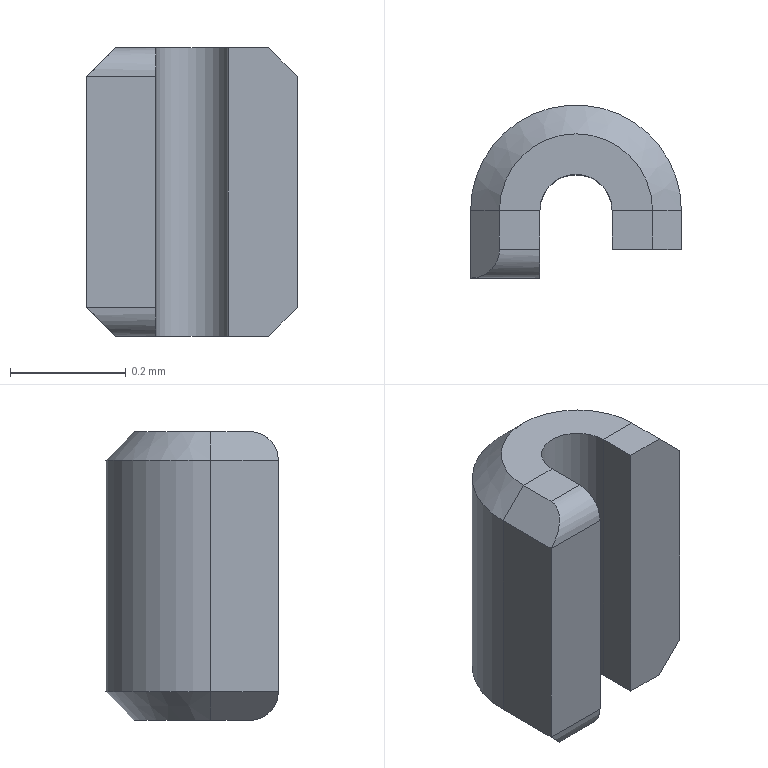Part | Creo | 1 solid | 22 faces | box 0.365 x 0.3 x 0.5 mm | volume 0.03234 mm3 | plane 16 | cylinder 4 | cone 2 | commonest cylinder face diameters 0.1 x2 0.125 x1 0.365 x1
STEP:
#1=CARTESIAN_POINT('',(0.,0.,0.));
#2=DIRECTION('',(0.,0.,1.));
#3=DIRECTION('',(1.,0.,0.));
#4=AXIS2_PLACEMENT_3D('',#1,#2,#3);
#5=CARTESIAN_POINT('',(-0.125,979.069,-1855.878));
#6=VERTEX_POINT('',#5);
#7=CARTESIAN_POINT('',(-0.195,979.069,-1855.878));
#8=VERTEX_POINT('',#7);
#9=CARTESIAN_POINT('',(-0.125,979.069,-1855.878));
#10=DIRECTION('',(-1.,0.,0.));
#11=VECTOR('',#10,0.07);
#12=LINE('',#9,#11);
#13=EDGE_CURVE('',#6,#8,#12,.T.);
#14=ORIENTED_EDGE('',*,*,#13,.F.);
#15=CARTESIAN_POINT('',(0.,979.069,-1855.878));
#16=VERTEX_POINT('',#15);
#17=CARTESIAN_POINT('',(-0.0625,979.069,-1855.878));
#18=DIRECTION('',(0.,0.,-1.));
#19=DIRECTION('',(-1.,0.,0.));
#20=AXIS2_PLACEMENT_3D('',#17,#18,#19);
#21=CIRCLE('',#20,0.0625);
#22=EDGE_CURVE('',#6,#16,#21,.T.);
#23=ORIENTED_EDGE('',*,*,#22,.T.);
#24=CARTESIAN_POINT('',(0.07,979.069,-1855.878));
#25=VERTEX_POINT('',#24);
#26=CARTESIAN_POINT('',(0.07,979.069,-1855.878));
#27=DIRECTION('',(-1.,0.,0.));
#28=VECTOR('',#27,0.07);
#29=LINE('',#26,#28);
#30=EDGE_CURVE('',#25,#16,#29,.T.);
#31=ORIENTED_EDGE('',*,*,#30,.F.);
#32=CARTESIAN_POINT('',(-0.0625,979.069,-1855.878));
#33=DIRECTION('',(0.,0.,1.));
#34=DIRECTION('',(1.,0.,0.));
#35=AXIS2_PLACEMENT_3D('',#32,#33,#34);
#36=CIRCLE('',#35,0.1325);
#37=EDGE_CURVE('',#25,#8,#36,.T.);
#38=ORIENTED_EDGE('',*,*,#37,.T.);
#39=EDGE_LOOP('',(#14,#23,#31,#38));
#40=FACE_OUTER_BOUND('',#39,.F.);
#41=CARTESIAN_POINT('',(-0.245,979.069,-1855.878));
#42=DIRECTION('',(0.,0.,-1.));
#43=DIRECTION('',(-1.,0.,0.));
#44=AXIS2_PLACEMENT_3D('',#41,#42,#43);
#45=PLANE('',#44);
#46=ADVANCED_FACE('',(#40),#45,.T.);
#47=CARTESIAN_POINT('',(-0.125,979.002,-1855.878));
#48=VERTEX_POINT('',#47);
#49=CARTESIAN_POINT('',(-0.125,979.002,-1855.878));
#50=DIRECTION('',(0.,1.,0.));
#51=VECTOR('',#50,0.0675);
#52=LINE('',#49,#51);
#53=EDGE_CURVE('',#48,#6,#52,.T.);
#54=ORIENTED_EDGE('',*,*,#53,.T.);
#55=ORIENTED_EDGE('',*,*,#13,.T.);
#56=CARTESIAN_POINT('',(-0.195,979.002,-1855.878));
#57=VERTEX_POINT('',#56);
#58=CARTESIAN_POINT('',(-0.195,979.069,-1855.878));
#59=DIRECTION('',(0.,-1.,0.));
#60=VECTOR('',#59,0.0675);
#61=LINE('',#58,#60);
#62=EDGE_CURVE('',#8,#57,#61,.T.);
#63=ORIENTED_EDGE('',*,*,#62,.T.);
#64=CARTESIAN_POINT('',(-0.125,979.002,-1855.878));
#65=DIRECTION('',(-1.,0.,0.));
#66=VECTOR('',#65,0.07);
#67=LINE('',#64,#66);
#68=EDGE_CURVE('',#48,#57,#67,.T.);
#69=ORIENTED_EDGE('',*,*,#68,.F.);
#70=EDGE_LOOP('',(#54,#55,#63,#69));
#71=FACE_OUTER_BOUND('',#70,.F.);
#72=CARTESIAN_POINT('',(0.,979.069,-1855.878));
#73=DIRECTION('',(0.,0.,-1.));
#74=DIRECTION('',(-1.,0.,0.));
#75=AXIS2_PLACEMENT_3D('',#72,#73,#74);
#76=PLANE('',#75);
#77=ADVANCED_FACE('',(#71),#76,.T.);
#78=CARTESIAN_POINT('',(-0.125,979.069,-1855.378));
#79=VERTEX_POINT('',#78);
#80=CARTESIAN_POINT('',(-0.125,979.002,-1855.378));
#81=VERTEX_POINT('',#80);
#82=CARTESIAN_POINT('',(-0.125,979.069,-1855.378));
#83=DIRECTION('',(0.,-1.,0.));
#84=VECTOR('',#83,0.0675);
#85=LINE('',#82,#84);
#86=EDGE_CURVE('',#79,#81,#85,.T.);
#87=ORIENTED_EDGE('',*,*,#86,.F.);
#88=CARTESIAN_POINT('',(-0.125,979.069,-1855.878));
#89=DIRECTION('',(0.,0.,1.));
#90=VECTOR('',#89,0.5);
#91=LINE('',#88,#90);
#92=EDGE_CURVE('',#6,#79,#91,.T.);
#93=ORIENTED_EDGE('',*,*,#92,.F.);
#94=ORIENTED_EDGE('',*,*,#53,.F.);
#95=CARTESIAN_POINT('',(-0.125,978.952,-1855.828));
#96=VERTEX_POINT('',#95);
#97=CARTESIAN_POINT('',(-0.125,979.002,-1855.828));
#98=DIRECTION('',(-1.,0.,0.));
#99=DIRECTION('',(0.,0.,-1.));
#100=AXIS2_PLACEMENT_3D('',#97,#98,#99);
#101=CIRCLE('',#100,0.05);
#102=EDGE_CURVE('',#48,#96,#101,.T.);
#103=ORIENTED_EDGE('',*,*,#102,.T.);
#104=CARTESIAN_POINT('',(-0.125,978.952,-1855.428));
#105=VERTEX_POINT('',#104);
#106=CARTESIAN_POINT('',(-0.125,978.952,-1855.828));
#107=DIRECTION('',(0.,0.,1.));
#108=VECTOR('',#107,0.4);
#109=LINE('',#106,#108);
#110=EDGE_CURVE('',#96,#105,#109,.T.);
#111=ORIENTED_EDGE('',*,*,#110,.T.);
#112=CARTESIAN_POINT('',(-0.125,979.002,-1855.428));
#113=DIRECTION('',(-1.,0.,0.));
#114=DIRECTION('',(0.,-1.,0.));
#115=AXIS2_PLACEMENT_3D('',#112,#113,#114);
#116=CIRCLE('',#115,0.05);
#117=EDGE_CURVE('',#105,#81,#116,.T.);
#118=ORIENTED_EDGE('',*,*,#117,.T.);
#119=EDGE_LOOP('',(#87,#93,#94,#103,#111,#118));
#120=FACE_OUTER_BOUND('',#119,.F.);
#121=CARTESIAN_POINT('',(-0.125,979.069,-1854.906));
#122=DIRECTION('',(1.,0.,0.));
#123=DIRECTION('',(0.,0.,-1.));
#124=AXIS2_PLACEMENT_3D('',#121,#122,#123);
#125=PLANE('',#124);
#126=ADVANCED_FACE('',(#120),#125,.T.);
#127=CARTESIAN_POINT('',(-0.195,979.002,-1855.378));
#128=VERTEX_POINT('',#127);
#129=CARTESIAN_POINT('',(-0.195,979.069,-1855.378));
#130=VERTEX_POINT('',#129);
#131=CARTESIAN_POINT('',(-0.195,979.002,-1855.378));
#132=DIRECTION('',(0.,1.,0.));
#133=VECTOR('',#132,0.0675);
#134=LINE('',#131,#133);
#135=EDGE_CURVE('',#128,#130,#134,.T.);
#136=ORIENTED_EDGE('',*,*,#135,.T.);
#137=CARTESIAN_POINT('',(-0.195,979.069,-1855.378));
#138=DIRECTION('',(1.,0.,0.));
#139=VECTOR('',#138,0.07);
#140=LINE('',#137,#139);
#141=EDGE_CURVE('',#130,#79,#140,.T.);
#142=ORIENTED_EDGE('',*,*,#141,.T.);
#143=ORIENTED_EDGE('',*,*,#86,.T.);
#144=CARTESIAN_POINT('',(-0.195,979.002,-1855.378));
#145=DIRECTION('',(1.,0.,0.));
#146=VECTOR('',#145,0.07);
#147=LINE('',#144,#146);
#148=EDGE_CURVE('',#128,#81,#147,.T.);
#149=ORIENTED_EDGE('',*,*,#148,.F.);
#150=EDGE_LOOP('',(#136,#142,#143,#149));
#151=FACE_OUTER_BOUND('',#150,.F.);
#152=CARTESIAN_POINT('',(-0.125,979.069,-1855.378));
#153=DIRECTION('',(0.,0.,-1.));
#154=DIRECTION('',(0.,1.,0.));
#155=AXIS2_PLACEMENT_3D('',#152,#153,#154);
#156=PLANE('',#155);
#157=ADVANCED_FACE('',(#151),#156,.F.);
#158=CARTESIAN_POINT('',(-0.245,979.069,-1855.428));
#159=VERTEX_POINT('',#158);
#160=CARTESIAN_POINT('',(-0.245,978.952,-1855.428));
#161=VERTEX_POINT('',#160);
#162=CARTESIAN_POINT('',(-0.245,979.069,-1855.428));
#163=DIRECTION('',(0.,-1.,0.));
#164=VECTOR('',#163,0.1175);
#165=LINE('',#162,#164);
#166=EDGE_CURVE('',#159,#161,#165,.T.);
#167=ORIENTED_EDGE('',*,*,#166,.F.);
#168=CARTESIAN_POINT('',(-0.195,979.069,-1855.378));
#169=DIRECTION('',(-0.7071,0.,-0.7071));
#170=VECTOR('',#169,0.07071);
#171=LINE('',#168,#170);
#172=EDGE_CURVE('',#130,#159,#171,.T.);
#173=ORIENTED_EDGE('',*,*,#172,.F.);
#174=ORIENTED_EDGE('',*,*,#135,.F.);
#175=CARTESIAN_POINT('',(-0.195,979.002,-1855.378));
#176=CARTESIAN_POINT('',(-0.195,978.997,-1855.378));
#177=CARTESIAN_POINT('',(-0.1964,978.988,-1855.38));
#178=CARTESIAN_POINT('',(-0.2002,978.979,-1855.384));
#179=CARTESIAN_POINT('',(-0.2052,978.971,-1855.389));
#180=CARTESIAN_POINT('',(-0.2133,978.962,-1855.397));
#181=CARTESIAN_POINT('',(-0.2256,978.954,-1855.409));
#182=CARTESIAN_POINT('',(-0.2379,978.952,-1855.421));
#183=CARTESIAN_POINT('',(-0.245,978.952,-1855.428));
#184=B_SPLINE_CURVE_WITH_KNOTS('',3,(#175,#176,#177,#178,#179,#180,#181,#182,#183),.UNSPECIFIED.,.F.,.F.,(4,1,1,1,1,1,4),(0.,0.125,0.25,0.375,0.5,0.75,1.),.UNSPECIFIED.);
#185=EDGE_CURVE('',#128,#161,#184,.T.);
#186=ORIENTED_EDGE('',*,*,#185,.T.);
#187=EDGE_LOOP('',(#167,#173,#174,#186));
#188=FACE_OUTER_BOUND('',#187,.F.);
#189=CARTESIAN_POINT('',(-0.245,979.069,-1855.428));
#190=DIRECTION('',(0.7071,0.,-0.7071));
#191=DIRECTION('',(-0.7071,0.,-0.7071));
#192=AXIS2_PLACEMENT_3D('',#189,#190,#191);
#193=PLANE('',#192);
#194=ADVANCED_FACE('',(#188),#193,.F.);
#195=CARTESIAN_POINT('',(-0.245,978.952,-1855.828));
#196=VERTEX_POINT('',#195);
#197=CARTESIAN_POINT('',(-0.245,978.952,-1855.828));
#198=DIRECTION('',(0.,0.,1.));
#199=VECTOR('',#198,0.4);
#200=LINE('',#197,#199);
#201=EDGE_CURVE('',#196,#161,#200,.T.);
#202=ORIENTED_EDGE('',*,*,#201,.F.);
#203=CARTESIAN_POINT('',(-0.245,979.069,-1855.828));
#204=VERTEX_POINT('',#203);
#205=CARTESIAN_POINT('',(-0.245,978.952,-1855.828));
#206=DIRECTION('',(0.,1.,0.));
#207=VECTOR('',#206,0.1175);
#208=LINE('',#205,#207);
#209=EDGE_CURVE('',#196,#204,#208,.T.);
#210=ORIENTED_EDGE('',*,*,#209,.T.);
#211=CARTESIAN_POINT('',(-0.245,979.069,-1855.428));
#212=DIRECTION('',(0.,0.,-1.));
#213=VECTOR('',#212,0.4);
#214=LINE('',#211,#213);
#215=EDGE_CURVE('',#159,#204,#214,.T.);
#216=ORIENTED_EDGE('',*,*,#215,.F.);
#217=ORIENTED_EDGE('',*,*,#166,.T.);
#218=EDGE_LOOP('',(#202,#210,#216,#217));
#219=FACE_OUTER_BOUND('',#218,.F.);
#220=CARTESIAN_POINT('',(-0.245,979.069,-1854.906));
#221=DIRECTION('',(1.,0.,0.));
#222=DIRECTION('',(0.,0.,-1.));
#223=AXIS2_PLACEMENT_3D('',#220,#221,#222);
#224=PLANE('',#223);
#225=ADVANCED_FACE('',(#219),#224,.F.);
#226=ORIENTED_EDGE('',*,*,#110,.F.);
#227=CARTESIAN_POINT('',(-0.245,978.952,-1855.828));
#228=DIRECTION('',(1.,0.,0.));
#229=VECTOR('',#228,0.12);
#230=LINE('',#227,#229);
#231=EDGE_CURVE('',#196,#96,#230,.T.);
#232=ORIENTED_EDGE('',*,*,#231,.F.);
#233=ORIENTED_EDGE('',*,*,#201,.T.);
#234=CARTESIAN_POINT('',(-0.125,978.952,-1855.428));
#235=DIRECTION('',(-1.,0.,0.));
#236=VECTOR('',#235,0.12);
#237=LINE('',#234,#236);
#238=EDGE_CURVE('',#105,#161,#237,.T.);
#239=ORIENTED_EDGE('',*,*,#238,.F.);
#240=EDGE_LOOP('',(#226,#232,#233,#239));
#241=FACE_OUTER_BOUND('',#240,.F.);
#242=CARTESIAN_POINT('',(-0.245,978.952,-1854.906));
#243=DIRECTION('',(0.,1.,0.));
#244=DIRECTION('',(0.,0.,1.));
#245=AXIS2_PLACEMENT_3D('',#242,#243,#244);
#246=PLANE('',#245);
#247=ADVANCED_FACE('',(#241),#246,.F.);
#248=CARTESIAN_POINT('',(-0.195,979.002,-1855.878));
#249=CARTESIAN_POINT('',(-0.195,978.997,-1855.878));
#250=CARTESIAN_POINT('',(-0.1964,978.988,-1855.877));
#251=CARTESIAN_POINT('',(-0.2002,978.979,-1855.873));
#252=CARTESIAN_POINT('',(-0.2052,978.971,-1855.868));
#253=CARTESIAN_POINT('',(-0.2133,978.962,-1855.86));
#254=CARTESIAN_POINT('',(-0.2256,978.954,-1855.848));
#255=CARTESIAN_POINT('',(-0.2379,978.952,-1855.835));
#256=CARTESIAN_POINT('',(-0.245,978.952,-1855.828));
#257=B_SPLINE_CURVE_WITH_KNOTS('',3,(#248,#249,#250,#251,#252,#253,#254,#255,#256),.UNSPECIFIED.,.F.,.F.,(4,1,1,1,1,1,4),(0.,0.125,0.25,0.375,0.5,0.75,1.),.UNSPECIFIED.);
#258=EDGE_CURVE('',#57,#196,#257,.T.);
#259=ORIENTED_EDGE('',*,*,#258,.T.);
#260=ORIENTED_EDGE('',*,*,#231,.T.);
#261=ORIENTED_EDGE('',*,*,#102,.F.);
#262=ORIENTED_EDGE('',*,*,#68,.T.);
#263=EDGE_LOOP('',(#259,#260,#261,#262));
#264=FACE_OUTER_BOUND('',#263,.F.);
#265=CARTESIAN_POINT('',(-0.245,979.002,-1855.828));
#266=DIRECTION('',(-1.,0.,0.));
#267=DIRECTION('',(0.,0.,1.));
#268=AXIS2_PLACEMENT_3D('',#265,#266,#267);
#269=CYLINDRICAL_SURFACE('',#268,0.05);
#270=ADVANCED_FACE('',(#264),#269,.T.);
#271=ORIENTED_EDGE('',*,*,#62,.F.);
#272=CARTESIAN_POINT('',(-0.245,979.069,-1855.828));
#273=DIRECTION('',(0.7071,0.,-0.7071));
#274=VECTOR('',#273,0.07071);
#275=LINE('',#272,#274);
#276=EDGE_CURVE('',#204,#8,#275,.T.);
#277=ORIENTED_EDGE('',*,*,#276,.F.);
#278=ORIENTED_EDGE('',*,*,#209,.F.);
#279=ORIENTED_EDGE('',*,*,#258,.F.);
#280=EDGE_LOOP('',(#271,#277,#278,#279));
#281=FACE_OUTER_BOUND('',#280,.F.);
#282=CARTESIAN_POINT('',(-0.245,979.069,-1855.828));
#283=DIRECTION('',(-0.7071,0.,-0.7071));
#284=DIRECTION('',(-0.7071,0.,0.7071));
#285=AXIS2_PLACEMENT_3D('',#282,#283,#284);
#286=PLANE('',#285);
#287=ADVANCED_FACE('',(#281),#286,.T.);
#288=ORIENTED_EDGE('',*,*,#276,.T.);
#289=ORIENTED_EDGE('',*,*,#37,.F.);
#290=CARTESIAN_POINT('',(0.12,979.069,-1855.828));
#291=VERTEX_POINT('',#290);
#292=CARTESIAN_POINT('',(0.07,979.069,-1855.878));
#293=DIRECTION('',(0.7071,0.,0.7071));
#294=VECTOR('',#293,0.07071);
#295=LINE('',#292,#294);
#296=EDGE_CURVE('',#25,#291,#295,.T.);
#297=ORIENTED_EDGE('',*,*,#296,.T.);
#298=CARTESIAN_POINT('',(-0.0625,979.069,-1855.828));
#299=DIRECTION('',(0.,0.,1.));
#300=DIRECTION('',(1.,0.,0.));
#301=AXIS2_PLACEMENT_3D('',#298,#299,#300);
#302=CIRCLE('',#301,0.1825);
#303=EDGE_CURVE('',#291,#204,#302,.T.);
#304=ORIENTED_EDGE('',*,*,#303,.T.);
#305=EDGE_LOOP('',(#288,#289,#297,#304));
#306=FACE_OUTER_BOUND('',#305,.F.);
#307=CARTESIAN_POINT('',(-0.0625,979.069,-1855.853));
#308=DIRECTION('',(0.,0.,1.));
#309=DIRECTION('',(1.,0.,0.));
#310=AXIS2_PLACEMENT_3D('',#307,#308,#309);
#311=CONICAL_SURFACE('',#310,0.1575,45.);
#312=ADVANCED_FACE('',(#306),#311,.T.);
#313=CARTESIAN_POINT('',(0.12,979.002,-1855.828));
#314=VERTEX_POINT('',#313);
#315=CARTESIAN_POINT('',(0.07,979.002,-1855.878));
#316=VERTEX_POINT('',#315);
#317=CARTESIAN_POINT('',(0.12,979.002,-1855.828));
#318=DIRECTION('',(-0.7071,0.,-0.7071));
#319=VECTOR('',#318,0.07071);
#320=LINE('',#317,#319);
#321=EDGE_CURVE('',#314,#316,#320,.T.);
#322=ORIENTED_EDGE('',*,*,#321,.F.);
#323=CARTESIAN_POINT('',(0.12,979.069,-1855.828));
#324=DIRECTION('',(0.,-1.,0.));
#325=VECTOR('',#324,0.0675);
#326=LINE('',#323,#325);
#327=EDGE_CURVE('',#291,#314,#326,.T.);
#328=ORIENTED_EDGE('',*,*,#327,.F.);
#329=ORIENTED_EDGE('',*,*,#296,.F.);
#330=CARTESIAN_POINT('',(0.07,979.002,-1855.878));
#331=DIRECTION('',(0.,1.,0.));
#332=VECTOR('',#331,0.0675);
#333=LINE('',#330,#332);
#334=EDGE_CURVE('',#316,#25,#333,.T.);
#335=ORIENTED_EDGE('',*,*,#334,.F.);
#336=EDGE_LOOP('',(#322,#328,#329,#335));
#337=FACE_OUTER_BOUND('',#336,.F.);
#338=CARTESIAN_POINT('',(0.12,979.002,-1855.828));
#339=DIRECTION('',(-0.7071,0.,0.7071));
#340=DIRECTION('',(0.7071,0.,0.7071));
#341=AXIS2_PLACEMENT_3D('',#338,#339,#340);
#342=PLANE('',#341);
#343=ADVANCED_FACE('',(#337),#342,.F.);
#344=CARTESIAN_POINT('',(0.12,979.002,-1855.428));
#345=VERTEX_POINT('',#344);
#346=CARTESIAN_POINT('',(0.12,979.002,-1855.828));
#347=DIRECTION('',(0.,0.,1.));
#348=VECTOR('',#347,0.4);
#349=LINE('',#346,#348);
#350=EDGE_CURVE('',#314,#345,#349,.T.);
#351=ORIENTED_EDGE('',*,*,#350,.F.);
#352=ORIENTED_EDGE('',*,*,#321,.T.);
#353=CARTESIAN_POINT('',(0.,979.002,-1855.878));
#354=VERTEX_POINT('',#353);
#355=CARTESIAN_POINT('',(0.07,979.002,-1855.878));
#356=DIRECTION('',(-1.,0.,0.));
#357=VECTOR('',#356,0.07);
#358=LINE('',#355,#357);
#359=EDGE_CURVE('',#316,#354,#358,.T.);
#360=ORIENTED_EDGE('',*,*,#359,.T.);
#361=CARTESIAN_POINT('',(0.,979.002,-1855.378));
#362=VERTEX_POINT('',#361);
#363=CARTESIAN_POINT('',(0.,979.002,-1855.878));
#364=DIRECTION('',(0.,0.,1.));
#365=VECTOR('',#364,0.5);
#366=LINE('',#363,#365);
#367=EDGE_CURVE('',#354,#362,#366,.T.);
#368=ORIENTED_EDGE('',*,*,#367,.T.);
#369=CARTESIAN_POINT('',(0.07,979.002,-1855.378));
#370=VERTEX_POINT('',#369);
#371=CARTESIAN_POINT('',(0.,979.002,-1855.378));
#372=DIRECTION('',(1.,0.,0.));
#373=VECTOR('',#372,0.07);
#374=LINE('',#371,#373);
#375=EDGE_CURVE('',#362,#370,#374,.T.);
#376=ORIENTED_EDGE('',*,*,#375,.T.);
#377=CARTESIAN_POINT('',(0.07,979.002,-1855.378));
#378=DIRECTION('',(0.7071,0.,-0.7071));
#379=VECTOR('',#378,0.07071);
#380=LINE('',#377,#379);
#381=EDGE_CURVE('',#370,#345,#380,.T.);
#382=ORIENTED_EDGE('',*,*,#381,.T.);
#383=EDGE_LOOP('',(#351,#352,#360,#368,#376,#382));
#384=FACE_OUTER_BOUND('',#383,.F.);
#385=CARTESIAN_POINT('',(0.,979.002,-1854.906));
#386=DIRECTION('',(0.,1.,0.));
#387=DIRECTION('',(0.,0.,1.));
#388=AXIS2_PLACEMENT_3D('',#385,#386,#387);
#389=PLANE('',#388);
#390=ADVANCED_FACE('',(#384),#389,.F.);
#391=CARTESIAN_POINT('',(0.12,979.069,-1855.428));
#392=VERTEX_POINT('',#391);
#393=CARTESIAN_POINT('',(0.12,979.069,-1855.828));
#394=DIRECTION('',(0.,0.,1.));
#395=VECTOR('',#394,0.4);
#396=LINE('',#393,#395);
#397=EDGE_CURVE('',#291,#392,#396,.T.);
#398=ORIENTED_EDGE('',*,*,#397,.F.);
#399=ORIENTED_EDGE('',*,*,#327,.T.);
#400=ORIENTED_EDGE('',*,*,#350,.T.);
#401=CARTESIAN_POINT('',(0.12,979.002,-1855.428));
#402=DIRECTION('',(0.,1.,0.));
#403=VECTOR('',#402,0.0675);
#404=LINE('',#401,#403);
#405=EDGE_CURVE('',#345,#392,#404,.T.);
#406=ORIENTED_EDGE('',*,*,#405,.T.);
#407=EDGE_LOOP('',(#398,#399,#400,#406));
#408=FACE_OUTER_BOUND('',#407,.F.);
#409=CARTESIAN_POINT('',(0.12,979.002,-1854.906));
#410=DIRECTION('',(-1.,0.,0.));
#411=DIRECTION('',(0.,0.,1.));
#412=AXIS2_PLACEMENT_3D('',#409,#410,#411);
#413=PLANE('',#412);
#414=ADVANCED_FACE('',(#408),#413,.F.);
#415=ORIENTED_EDGE('',*,*,#215,.T.);
#416=ORIENTED_EDGE('',*,*,#303,.F.);
#417=ORIENTED_EDGE('',*,*,#397,.T.);
#418=CARTESIAN_POINT('',(-0.0625,979.069,-1855.428));
#419=DIRECTION('',(0.,0.,-1.));
#420=DIRECTION('',(-1.,0.,0.));
#421=AXIS2_PLACEMENT_3D('',#418,#419,#420);
#422=CIRCLE('',#421,0.1825);
#423=EDGE_CURVE('',#159,#392,#422,.T.);
#424=ORIENTED_EDGE('',*,*,#423,.F.);
#425=EDGE_LOOP('',(#415,#416,#417,#424));
#426=FACE_OUTER_BOUND('',#425,.F.);
#427=CARTESIAN_POINT('',(-0.0625,979.069,-1854.906));
#428=DIRECTION('',(0.,0.,-1.));
#429=DIRECTION('',(-1.,0.,0.));
#430=AXIS2_PLACEMENT_3D('',#427,#428,#429);
#431=CYLINDRICAL_SURFACE('',#430,0.1825);
#432=ADVANCED_FACE('',(#426),#431,.T.);
#433=ORIENTED_EDGE('',*,*,#172,.T.);
#434=ORIENTED_EDGE('',*,*,#423,.T.);
#435=CARTESIAN_POINT('',(0.07,979.069,-1855.378));
#436=VERTEX_POINT('',#435);
#437=CARTESIAN_POINT('',(0.12,979.069,-1855.428));
#438=DIRECTION('',(-0.7071,0.,0.7071));
#439=VECTOR('',#438,0.07071);
#440=LINE('',#437,#439);
#441=EDGE_CURVE('',#392,#436,#440,.T.);
#442=ORIENTED_EDGE('',*,*,#441,.T.);
#443=CARTESIAN_POINT('',(-0.0625,979.069,-1855.378));
#444=DIRECTION('',(0.,0.,-1.));
#445=DIRECTION('',(-1.,0.,0.));
#446=AXIS2_PLACEMENT_3D('',#443,#444,#445);
#447=CIRCLE('',#446,0.1325);
#448=EDGE_CURVE('',#130,#436,#447,.T.);
#449=ORIENTED_EDGE('',*,*,#448,.F.);
#450=EDGE_LOOP('',(#433,#434,#442,#449));
#451=FACE_OUTER_BOUND('',#450,.F.);
#452=CARTESIAN_POINT('',(-0.0625,979.069,-1855.403));
#453=DIRECTION('',(0.,0.,-1.));
#454=DIRECTION('',(-1.,0.,0.));
#455=AXIS2_PLACEMENT_3D('',#452,#453,#454);
#456=CONICAL_SURFACE('',#455,0.1575,45.);
#457=ADVANCED_FACE('',(#451),#456,.T.);
#458=ORIENTED_EDGE('',*,*,#441,.F.);
#459=ORIENTED_EDGE('',*,*,#405,.F.);
#460=ORIENTED_EDGE('',*,*,#381,.F.);
#461=CARTESIAN_POINT('',(0.07,979.069,-1855.378));
#462=DIRECTION('',(0.,-1.,0.));
#463=VECTOR('',#462,0.0675);
#464=LINE('',#461,#463);
#465=EDGE_CURVE('',#436,#370,#464,.T.);
#466=ORIENTED_EDGE('',*,*,#465,.F.);
#467=EDGE_LOOP('',(#458,#459,#460,#466));
#468=FACE_OUTER_BOUND('',#467,.F.);
#469=CARTESIAN_POINT('',(0.12,979.002,-1855.428));
#470=DIRECTION('',(-0.7071,0.,-0.7071));
#471=DIRECTION('',(-0.7071,0.,0.7071));
#472=AXIS2_PLACEMENT_3D('',#469,#470,#471);
#473=PLANE('',#472);
#474=ADVANCED_FACE('',(#468),#473,.F.);
#475=ORIENTED_EDGE('',*,*,#375,.F.);
#476=CARTESIAN_POINT('',(0.,979.069,-1855.378));
#477=VERTEX_POINT('',#476);
#478=CARTESIAN_POINT('',(0.,979.002,-1855.378));
#479=DIRECTION('',(0.,1.,0.));
#480=VECTOR('',#479,0.0675);
#481=LINE('',#478,#480);
#482=EDGE_CURVE('',#362,#477,#481,.T.);
#483=ORIENTED_EDGE('',*,*,#482,.T.);
#484=CARTESIAN_POINT('',(0.,979.069,-1855.378));
#485=DIRECTION('',(1.,0.,0.));
#486=VECTOR('',#485,0.07);
#487=LINE('',#484,#486);
#488=EDGE_CURVE('',#477,#436,#487,.T.);
#489=ORIENTED_EDGE('',*,*,#488,.T.);
#490=ORIENTED_EDGE('',*,*,#465,.T.);
#491=EDGE_LOOP('',(#475,#483,#489,#490));
#492=FACE_OUTER_BOUND('',#491,.F.);
#493=CARTESIAN_POINT('',(0.12,979.002,-1855.378));
#494=DIRECTION('',(0.,0.,-1.));
#495=DIRECTION('',(0.,-1.,0.));
#496=AXIS2_PLACEMENT_3D('',#493,#494,#495);
#497=PLANE('',#496);
#498=ADVANCED_FACE('',(#492),#497,.F.);
#499=ORIENTED_EDGE('',*,*,#367,.F.);
#500=CARTESIAN_POINT('',(0.,979.069,-1855.878));
#501=DIRECTION('',(0.,-1.,0.));
#502=VECTOR('',#501,0.0675);
#503=LINE('',#500,#502);
#504=EDGE_CURVE('',#16,#354,#503,.T.);
#505=ORIENTED_EDGE('',*,*,#504,.F.);
#506=CARTESIAN_POINT('',(0.,979.069,-1855.378));
#507=DIRECTION('',(0.,0.,-1.));
#508=VECTOR('',#507,0.5);
#509=LINE('',#506,#508);
#510=EDGE_CURVE('',#477,#16,#509,.T.);
#511=ORIENTED_EDGE('',*,*,#510,.F.);
#512=ORIENTED_EDGE('',*,*,#482,.F.);
#513=EDGE_LOOP('',(#499,#505,#511,#512));
#514=FACE_OUTER_BOUND('',#513,.F.);
#515=CARTESIAN_POINT('',(0.,979.002,-1854.906));
#516=DIRECTION('',(-1.,0.,0.));
#517=DIRECTION('',(0.,0.,1.));
#518=AXIS2_PLACEMENT_3D('',#515,#516,#517);
#519=PLANE('',#518);
#520=ADVANCED_FACE('',(#514),#519,.T.);
#521=ORIENTED_EDGE('',*,*,#30,.T.);
#522=ORIENTED_EDGE('',*,*,#504,.T.);
#523=ORIENTED_EDGE('',*,*,#359,.F.);
#524=ORIENTED_EDGE('',*,*,#334,.T.);
#525=EDGE_LOOP('',(#521,#522,#523,#524));
#526=FACE_OUTER_BOUND('',#525,.F.);
#527=CARTESIAN_POINT('',(-0.0625,979.069,-1855.878));
#528=DIRECTION('',(0.,0.,1.));
#529=DIRECTION('',(1.,0.,0.));
#530=AXIS2_PLACEMENT_3D('',#527,#528,#529);
#531=PLANE('',#530);
#532=ADVANCED_FACE('',(#526),#531,.F.);
#533=ORIENTED_EDGE('',*,*,#510,.T.);
#534=ORIENTED_EDGE('',*,*,#22,.F.);
#535=ORIENTED_EDGE('',*,*,#92,.T.);
#536=CARTESIAN_POINT('',(-0.0625,979.069,-1855.378));
#537=DIRECTION('',(0.,0.,1.));
#538=DIRECTION('',(1.,0.,0.));
#539=AXIS2_PLACEMENT_3D('',#536,#537,#538);
#540=CIRCLE('',#539,0.0625);
#541=EDGE_CURVE('',#477,#79,#540,.T.);
#542=ORIENTED_EDGE('',*,*,#541,.F.);
#543=EDGE_LOOP('',(#533,#534,#535,#542));
#544=FACE_OUTER_BOUND('',#543,.F.);
#545=CARTESIAN_POINT('',(-0.0625,979.069,-1854.906));
#546=DIRECTION('',(0.,0.,-1.));
#547=DIRECTION('',(-1.,0.,0.));
#548=AXIS2_PLACEMENT_3D('',#545,#546,#547);
#549=CYLINDRICAL_SURFACE('',#548,0.0625);
#550=ADVANCED_FACE('',(#544),#549,.F.);
#551=ORIENTED_EDGE('',*,*,#488,.F.);
#552=ORIENTED_EDGE('',*,*,#541,.T.);
#553=ORIENTED_EDGE('',*,*,#141,.F.);
#554=ORIENTED_EDGE('',*,*,#448,.T.);
#555=EDGE_LOOP('',(#551,#552,#553,#554));
#556=FACE_OUTER_BOUND('',#555,.F.);
#557=CARTESIAN_POINT('',(-0.0625,979.069,-1855.378));
#558=DIRECTION('',(0.,0.,1.));
#559=DIRECTION('',(1.,0.,0.));
#560=AXIS2_PLACEMENT_3D('',#557,#558,#559);
#561=PLANE('',#560);
#562=ADVANCED_FACE('',(#556),#561,.T.);
#563=ORIENTED_EDGE('',*,*,#117,.F.);
#564=ORIENTED_EDGE('',*,*,#238,.T.);
#565=ORIENTED_EDGE('',*,*,#185,.F.);
#566=ORIENTED_EDGE('',*,*,#148,.T.);
#567=EDGE_LOOP('',(#563,#564,#565,#566));
#568=FACE_OUTER_BOUND('',#567,.F.);
#569=CARTESIAN_POINT('',(-0.245,979.002,-1855.428));
#570=DIRECTION('',(-1.,0.,0.));
#571=DIRECTION('',(0.,0.,1.));
#572=AXIS2_PLACEMENT_3D('',#569,#570,#571);
#573=CYLINDRICAL_SURFACE('',#572,0.05);
#574=ADVANCED_FACE('',(#568),#573,.T.);
#575=CLOSED_SHELL('',(#46,#77,#126,#157,#194,#225,#247,#270,#287,#312,#343,#390,#414,#432,#457,#474,#498,#520,#532,#550,#562,#574));
#576=MANIFOLD_SOLID_BREP('',#575);
#577=(LENGTH_UNIT()NAMED_UNIT(*)SI_UNIT(.MILLI.,.METRE.));
#578=UNCERTAINTY_MEASURE_WITH_UNIT(LENGTH_MEASURE(0.00006879),#577,'','');
#579=(NAMED_UNIT(*)PLANE_ANGLE_UNIT()SI_UNIT($,.RADIAN.));
#580=PLANE_ANGLE_MEASURE_WITH_UNIT(PLANE_ANGLE_MEASURE(0.01745),#579);
#581=(CONVERSION_BASED_UNIT('DEGREE',#580)NAMED_UNIT(*)PLANE_ANGLE_UNIT());
#582=(NAMED_UNIT(*)SI_UNIT($,.STERADIAN.)SOLID_ANGLE_UNIT());
#583=(GEOMETRIC_REPRESENTATION_CONTEXT(3)GLOBAL_UNCERTAINTY_ASSIGNED_CONTEXT((#578))GLOBAL_UNIT_ASSIGNED_CONTEXT((#577,#581,#582))REPRESENTATION_CONTEXT('',''));
#584=ADVANCED_BREP_SHAPE_REPRESENTATION('',(#4,#576),#583);